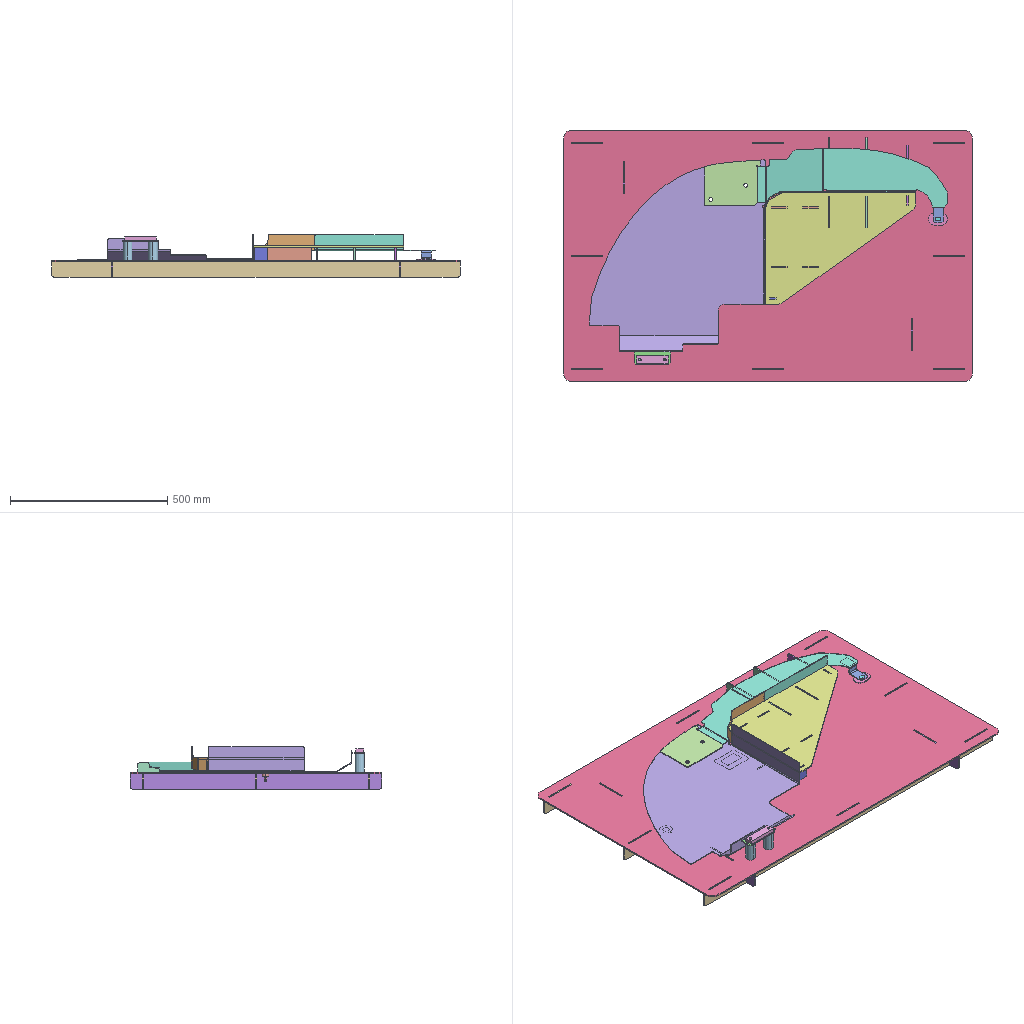Assembly | SolidWorks | 13 different items | 19 placed | box 1300 x 800 x 137 mm
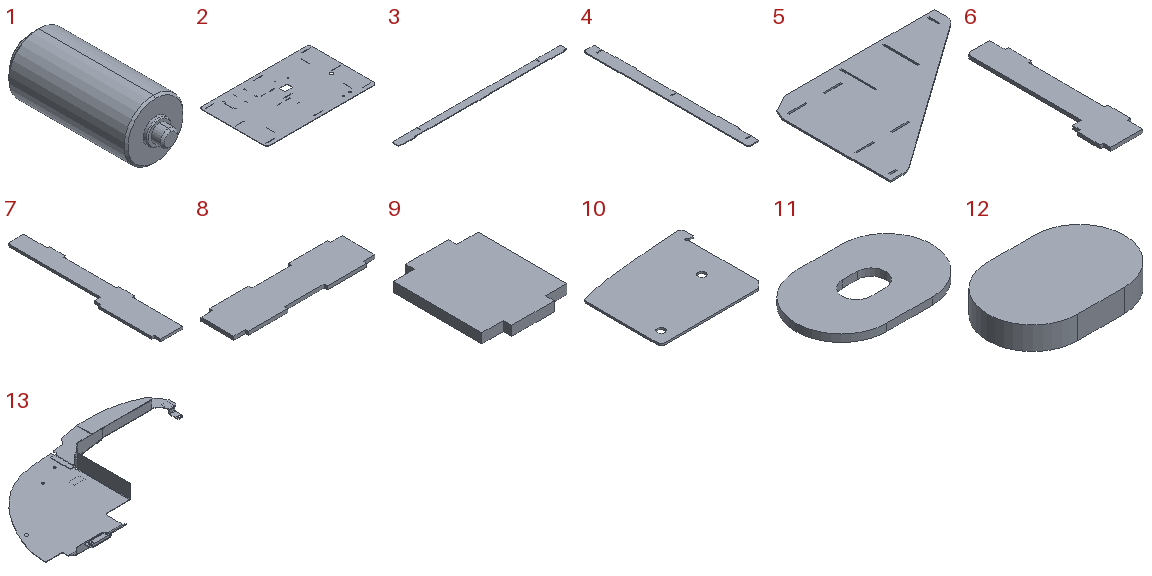Parts list (item | quantity | size | volume | features):
1 | x2 | 30 x 72 x 30 mm | 44332 mm3 | features Chamfer 2, Revolution 1
2 | x1 | 1300 x 800 x 4.5 mm | 4605383 mm3 | features FlatPattern 1, SMBaseFlange 1, SheetMetal 1
3 | x3 | 1300 x 54 x 4.5 mm | 296674 mm3 | features FlatPattern 1, SMBaseFlange 1, SheetMetal 1
4 | x2 | 54 x 800 x 4.5 mm | 181888 mm3 | features FlatPattern 1, SMBaseFlange 1, SheetMetal 1
5 | x1 | 479.97 x 356 x 4.5 mm | 459091 mm3 | features FlatPattern 1, SMBaseFlange 1, SheetMetal 1
6 | x1 | 49.8 x 200 x 4.5 mm | 31251 mm3 | features FlatPattern 1, SMBaseFlange 1, SheetMetal 1
7 | x2 | 49.8 x 300 x 4.5 mm | 49993 mm3 | features FlatPattern 1, SMBaseFlange 1, SheetMetal 1
8 | x2 | 180 x 49.8 x 4.5 mm | 37458 mm3 | features FlatPattern 1, SMBaseFlange 1, SheetMetal 1
9 | x1 | 40 x 49.8 x 4.5 mm | 8244 mm3 | features FlatPattern 1, SMBaseFlange 1, SheetMetal 1
10 | x1 | 177.818 x 145.585 x 3.2 mm | 73602 mm3 | features FlatPattern 1, SMBaseFlange 1, SheetMetal 1
11 | x1 | 60 x 40 x 3.2 mm | 5929 mm3 | features FlatPattern 1, SMBaseFlange 1, SheetMetal 1
12 | x1 | 19 x 12.5 x 3.2 mm | 652.699 mm3 | features FlatPattern 1, SMBaseFlange 1, SheetMetal 1
13 | x1 | 1139 x 687.3 x 112.3 mm | 932839 mm3 | features MBimport 1
Mates (type | each side: item.copy, entity, surface, feature):
InPlace | 13.1 face plane | 2.1 plane
InPlace | 1.1 plane | assembly plane
InPlace | 13.1 face plane | 5.1 plane
InPlace | 6.1 plane | assembly plane
InPlace | 7.1 plane | assembly plane
InPlace | 8.1 plane | assembly plane
InPlace | 9.1 plane | assembly plane
InPlace | 13.1 face plane | 10.1 plane
InPlace | 2.1 face plane Base-Flange1 | 11.1 plane
InPlace | 11.1 face plane Base-Flange1 | 12.1 plane
InPlace | 3.1 plane | assembly plane
InPlace | 4.1 plane | assembly plane